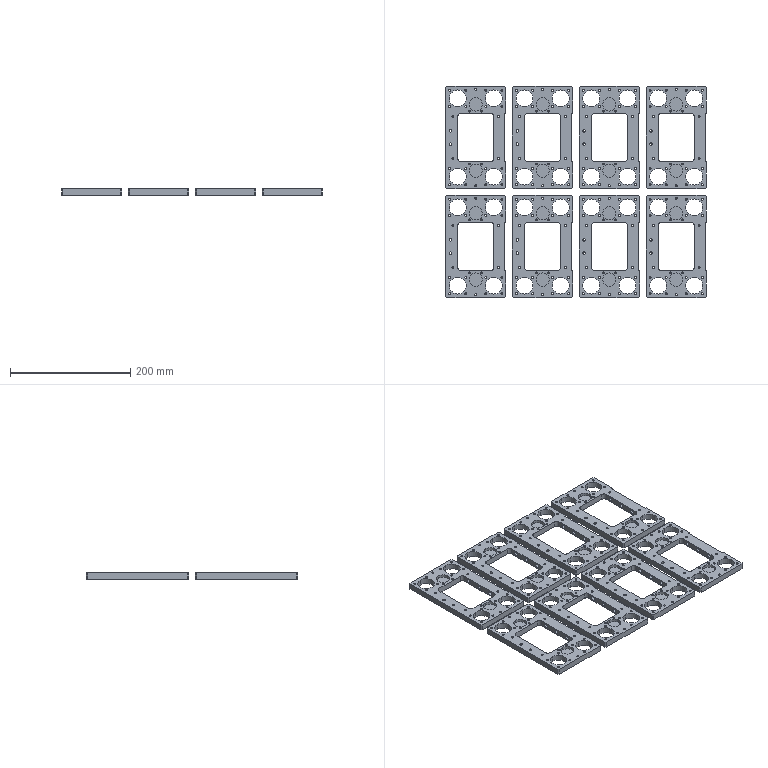NC program | NX | posted with a generic post | part box 433 x 351 x 10 mm
Lines 1 to 529 of 15742:
N10 G17 G21 G94 G90
(DRILLING , TOOL : D6A45)
N12 T01 M6
N14 G54
N16 G17 G0 G90 X-17.5 Y-55.5 B0. C0. S5000 M3
N18 G43 Z30. H1
N20 G94 G81 G98 Z-1. F350. R3.
N22 X-12.065 Y-38.935
N24 X-25.5 Y-25.5
N26 X-12.065 Y-12.065
N28 Y12.065
N30 X12.065
N32 Y-12.065
N34 X38.935
N36 Y12.065
N38 X55.5 Y10.5
N40 X72.065 Y12.065
N42 X85.5 Y25.5
N44 X72.065 Y38.935
N46 X65.5 Y46.5
N48 X55.5 Y35.5
N50 X45.5 Y46.5
N52 X38.935 Y38.935
N54 X25.5 Y25.5
N56 X12.065 Y38.935
N58 X-12.065
N60 X-17.5 Y55.5
N62 X17.5
N64 X13.5 Y79.5
N66 Y101.5
N68 X-17.5 Y125.5
N70 X-12.065 Y142.065
N72 X-25.5 Y155.5
N74 X-38.935 Y142.065
N76 X-45.5 Y134.5
N78 X-55.5 Y145.5
N80 X-65.5 Y134.5
N82 X-72.065 Y142.065
N84 Y168.935
N86 X-55.5 Y170.5
N88 X-38.935 Y168.935
N90 X-12.065
N92 X12.065
N94 X25.5 Y155.5
N96 X12.065 Y142.065
N98 X17.5 Y125.5
N100 X45.5 Y134.5
N102 X38.935 Y142.065
N104 Y168.935
N106 X55.5 Y170.5
N108 X72.065 Y168.935
N110 X55.5 Y145.5
N112 X65.5 Y134.5
N114 X72.065 Y142.065
N116 X93.5 Y125.5
N118 X98.935 Y142.065
N120 X85.5 Y155.5
N122 X98.935 Y168.935
N124 X123.065
N126 X149.935
N128 X166.5 Y170.5
N130 X183.065 Y168.935
N132 X196.5 Y155.5
N134 X209.935 Y168.935
N136 Y142.065
N138 X204.5 Y125.5
N140 X183.065 Y142.065
N142 X176.5 Y134.5
N144 X166.5 Y145.5
N146 X156.5 Y134.5
N148 X149.935 Y142.065
N150 X136.5 Y155.5
N152 X123.065 Y142.065
N154 X128.5 Y125.5
N156 X124.5 Y101.5
N158 Y79.5
N160 X128.5 Y55.5
N162 X123.065 Y38.935
N164 X93.5 Y55.5
N166 X98.935 Y38.935
N168 Y12.065
N170 X123.065
N172 X136.5 Y25.5
N174 X149.935 Y38.935
N176 X156.5 Y46.5
N178 X166.5 Y35.5
N180 X176.5 Y46.5
N182 X183.065 Y38.935
N184 X204.5 Y55.5
N186 X209.935 Y38.935
N188 X196.5 Y25.5
N190 X183.065 Y12.065
N192 X209.935
N194 Y-12.065
N196 X196.5 Y-25.5
N198 X209.935 Y-38.935
N200 X204.5 Y-55.5
N202 X183.065 Y-38.935
N204 X176.5 Y-46.5
N206 X166.5 Y-35.5
N208 X156.5 Y-46.5
N210 X149.935 Y-38.935
N212 X166.5 Y-10.5
N214 X183.065 Y-12.065
N216 X166.5 Y10.5
N218 X149.935 Y12.065
N220 Y-12.065
N222 X136.5 Y-25.5
N224 X123.065 Y-12.065
N226 X98.935
N228 X85.5 Y-25.5
N230 X72.065 Y-12.065
N232 X55.5 Y-10.5
N234 Y-35.5
N236 X72.065 Y-38.935
N238 X65.5 Y-46.5
N240 X45.5
N242 X38.935 Y-38.935
N244 X25.5 Y-25.5
N246 X12.065 Y-38.935
N248 X17.5 Y-55.5
N250 X13.5 Y-79.5
N252 Y-101.5
N254 X17.5 Y-125.5
N256 X12.065 Y-142.065
N258 X-12.065
N260 X-17.5 Y-125.5
N262 X-38.935 Y-142.065
N264 X-45.5 Y-134.5
N266 X-55.5 Y-145.5
N268 X-65.5 Y-134.5
N270 X-72.065 Y-142.065
N272 X-98.935
N274 X-93.5 Y-125.5
N276 X-97.5 Y-101.5
N278 Y-79.5
N280 X-93.5 Y-55.5
N282 X-98.935 Y-38.935
N284 X-85.5 Y-25.5
N286 X-72.065 Y-38.935
N288 X-65.5 Y-46.5
N290 X-55.5 Y-35.5
N292 X-45.5 Y-46.5
N294 X-38.935 Y-38.935
N296 Y-12.065
N298 X-55.5 Y-10.5
N300 X-72.065 Y-12.065
N302 Y12.065
N304 X-55.5 Y10.5
N306 X-38.935 Y12.065
N308 X-25.5 Y25.5
N310 X-38.935 Y38.935
N312 X-45.5 Y46.5
N314 X-55.5 Y35.5
N316 X-65.5 Y46.5
N318 X-72.065 Y38.935
N320 X-85.5 Y25.5
N322 X-98.935 Y12.065
N324 Y-12.065
N326 X-123.065
N328 Y12.065
N330 X-136.5 Y25.5
N332 X-149.935 Y12.065
N334 X-166.5 Y10.5
N336 Y35.5
N338 X-183.065 Y38.935
N340 X-176.5 Y46.5
N342 X-156.5
N344 X-149.935 Y38.935
N346 X-128.5 Y55.5
N348 X-123.065 Y38.935
N350 X-98.935
N352 X-93.5 Y55.5
N354 X-97.5 Y79.5
N356 Y101.5
N358 X-93.5 Y125.5
N360 X-98.935 Y142.065
N362 X-85.5 Y155.5
N364 X-98.935 Y168.935
N366 X-123.065
N368 Y142.065
N370 X-128.5 Y125.5
N372 X-156.5 Y134.5
N374 X-176.5
N376 X-183.065 Y142.065
N378 X-166.5 Y145.5
N380 X-149.935 Y142.065
N382 X-136.5 Y155.5
N384 X-149.935 Y168.935
N386 X-166.5 Y170.5
N388 X-183.065 Y168.935
N390 X-196.5 Y155.5
N392 X-209.935 Y168.935
N394 Y142.065
N396 X-204.5 Y125.5
N398 X-208.5 Y101.5
N400 Y79.5
N402 X-204.5 Y55.5
N404 X-209.935 Y38.935
N406 Y12.065
N408 X-196.5 Y25.5
N410 X-183.065 Y12.065
N412 Y-12.065
N414 X-166.5 Y-10.5
N416 X-149.935 Y-12.065
N418 X-136.5 Y-25.5
N420 X-123.065 Y-38.935
N422 X-128.5 Y-55.5
N424 X-149.935 Y-38.935
N426 X-156.5 Y-46.5
N428 X-166.5 Y-35.5
N430 X-176.5 Y-46.5
N432 X-183.065 Y-38.935
N434 X-196.5 Y-25.5
N436 X-209.935 Y-12.065
N438 Y-38.935
N440 X-204.5 Y-55.5
N442 X-208.5 Y-79.5
N444 Y-101.5
N446 X-204.5 Y-125.5
N448 X-209.935 Y-142.065
N450 Y-168.935
N452 X-196.5 Y-155.5
N454 X-183.065 Y-168.935
N456 X-166.5 Y-170.5
N458 X-183.065 Y-142.065
N460 X-176.5 Y-134.5
N462 X-166.5 Y-145.5
N464 X-156.5 Y-134.5
N466 X-149.935 Y-142.065
N468 X-128.5 Y-125.5
N470 X-123.065 Y-142.065
N472 X-136.5 Y-155.5
N474 X-149.935 Y-168.935
N476 X-123.065
N478 X-98.935
N480 X-85.5 Y-155.5
N482 X-72.065 Y-168.935
N484 X-55.5 Y-170.5
N486 X-38.935 Y-168.935
N488 X-25.5 Y-155.5
N490 X-12.065 Y-168.935
N492 X12.065
N494 X25.5 Y-155.5
N496 X38.935 Y-142.065
N498 X45.5 Y-134.5
N500 X55.5 Y-145.5
N502 X38.935 Y-168.935
N504 X55.5 Y-170.5
N506 X72.065 Y-168.935
N508 X65.5 Y-134.5
N510 X72.065 Y-142.065
N512 X85.5 Y-155.5
N514 X98.935 Y-168.935
N516 X123.065
N518 X149.935
N520 X166.5 Y-170.5
N522 X183.065 Y-168.935
N524 X209.935
N526 X196.5 Y-155.5
N528 X209.935 Y-142.065
N530 X204.5 Y-125.5
N532 X183.065 Y-142.065
N534 X176.5 Y-134.5
N536 X166.5 Y-145.5
N538 X156.5 Y-134.5
N540 X149.935 Y-142.065
N542 X136.5 Y-155.5
N544 X123.065 Y-142.065
N546 X98.935
N548 X93.5 Y-125.5
N550 X128.5
N552 X124.5 Y-101.5
N554 Y-79.5
N556 X128.5 Y-55.5
N558 X123.065 Y-38.935
N560 X98.935
N562 X93.5 Y-55.5
N564 G80
N566 G0 X93.5 Y-55.5 Z30.
N568 M5
(DRILLING_COPY , TOOL : 3.3ZT)
N570 T03 M6
N572 G54
N574 G17 G0 G90 X-209.935 Y168.935 B0. C0. S2000 M3
N576 G43 Z30. H3
N578 G94 G83 G98 Z-12.491 F200. Q2. R3.
N580 X-183.065
N582 X-166.5 Y170.5
N584 X-149.935 Y168.935
N586 X-123.065
N588 X-98.935
N590 X-72.065
N592 X-55.5 Y170.5
N594 X-38.935 Y168.935
N596 X-12.065
N598 X12.065
N600 X38.935
N602 X55.5 Y170.5
N604 X72.065 Y168.935
N606 X98.935
N608 X123.065
N610 X149.935
N612 X166.5 Y170.5
N614 X183.065 Y168.935
N616 X209.935
N618 Y142.065
N620 X204.5 Y125.5
N622 X183.065 Y142.065
N624 X176.5 Y134.5
N626 X156.5
N628 X149.935 Y142.065
N630 X128.5 Y125.5
N632 X123.065 Y142.065
N634 X98.935
N636 X93.5 Y125.5
N638 X72.065 Y142.065
N640 X65.5 Y134.5
N642 X45.5
N644 X38.935 Y142.065
N646 X17.5 Y125.5
N648 X12.065 Y142.065
N650 X-12.065
N652 X-17.5 Y125.5
N654 X-38.935 Y142.065
N656 X-45.5 Y134.5
N658 X-65.5
N660 X-72.065 Y142.065
N662 X-93.5 Y125.5
N664 X-98.935 Y142.065
N666 X-123.065
N668 X-128.5 Y125.5
N670 X-149.935 Y142.065
N672 X-156.5 Y134.5
N674 X-176.5
N676 X-183.065 Y142.065
N678 X-209.935
N680 X-204.5 Y125.5
N682 X-176.5 Y46.5
N684 X-183.065 Y38.935
N686 X-204.5 Y55.5
N688 X-209.935 Y38.935
N690 Y12.065
N692 Y-12.065
N694 Y-38.935
N696 X-204.5 Y-55.5
N698 X-183.065 Y-38.935
N700 X-176.5 Y-46.5
N702 X-156.5
N704 X-149.935 Y-38.935
N706 Y-12.065
N708 X-166.5 Y-10.5
N710 X-183.065 Y-12.065
N712 Y12.065
N714 X-166.5 Y10.5
N716 X-149.935 Y12.065
N718 Y38.935
N720 X-156.5 Y46.5
N722 X-128.5 Y55.5
N724 X-123.065 Y38.935
N726 Y12.065
N728 X-98.935
N730 X-72.065 Y-12.065
N732 X-55.5 Y-10.5
N734 X-38.935 Y-12.065
N736 Y12.065
N738 X-55.5 Y10.5
N740 X-72.065 Y12.065
N742 X-98.935 Y38.935
N744 X-93.5 Y55.5
N746 X-72.065 Y38.935
N748 X-65.5 Y46.5
N750 X-45.5
N752 X-38.935 Y38.935
N754 X-17.5 Y55.5
N756 X-12.065 Y38.935
N758 Y12.065
N760 X12.065
N762 Y38.935
N764 X17.5 Y55.5
N766 X38.935 Y38.935
N768 X45.5 Y46.5
N770 X65.5
N772 X72.065 Y38.935
N774 X93.5 Y55.5
N776 X98.935 Y38.935
N778 X123.065
N780 X128.5 Y55.5
N782 X149.935 Y38.935
N784 X156.5 Y46.5
N786 X176.5
N788 X183.065 Y38.935
N790 X204.5 Y55.5
N792 X209.935 Y38.935
N794 Y12.065
N796 Y-12.065
N798 Y-38.935
N800 X204.5 Y-55.5
N802 X183.065 Y-38.935
N804 X176.5 Y-46.5
N806 X156.5
N808 X149.935 Y-38.935
N810 Y-12.065
N812 X166.5 Y-10.5
N814 X183.065 Y-12.065
N816 Y12.065
N818 X166.5 Y10.5
N820 X149.935 Y12.065
N822 X123.065
N824 Y-12.065
N826 Y-38.935
N828 X128.5 Y-55.5
N830 X98.935 Y-38.935
N832 X93.5 Y-55.5
N834 X72.065 Y-38.935
N836 X65.5 Y-46.5
N838 X45.5
N840 X38.935 Y-38.935
N842 Y-12.065
N844 X55.5 Y-10.5
N846 X72.065 Y-12.065
N848 X98.935
N850 Y12.065
N852 X72.065
N854 X55.5 Y10.5
N856 X38.935 Y12.065
N858 X12.065 Y-12.065
N860 X-12.065
N862 X12.065 Y-38.935
N864 X17.5 Y-55.5
N866 X-12.065 Y-38.935
N868 X-17.5 Y-55.5
N870 X-38.935 Y-38.935
N872 X-45.5 Y-46.5
N874 X-65.5
N876 X-72.065 Y-38.935
N878 X-93.5 Y-55.5
N880 X-98.935 Y-38.935
N882 Y-12.065
N884 X-123.065
N886 Y-38.935
N888 X-128.5 Y-55.5
N890 Y-125.5
N892 X-123.065 Y-142.065
N894 X-98.935
N896 X-93.5 Y-125.5
N898 X-72.065 Y-142.065
N900 X-65.5 Y-134.5
N902 X-45.5
N904 X-38.935 Y-142.065
N906 X-17.5 Y-125.5
N908 X-12.065 Y-142.065
N910 X12.065
N912 X17.5 Y-125.5
N914 X38.935 Y-142.065
N916 X45.5 Y-134.5
N918 X65.5
N920 X72.065 Y-142.065
N922 X93.5 Y-125.5
N924 X98.935 Y-142.065
N926 X123.065
N928 X128.5 Y-125.5
N930 X149.935 Y-142.065
N932 X156.5 Y-134.5
N934 X176.5
N936 X183.065 Y-142.065
N938 X204.5 Y-125.5
N940 X209.935 Y-142.065
N942 Y-168.935
N944 X183.065
N946 X166.5 Y-170.5
N948 X149.935 Y-168.935
N950 X123.065
N952 X98.935
N954 X72.065
N956 X55.5 Y-170.5
N958 X38.935 Y-168.935
N960 X12.065
N962 X-12.065
N964 X-38.935
N966 X-55.5 Y-170.5
N968 X-72.065 Y-168.935
N970 X-98.935
N972 X-123.065
N974 X-149.935
N976 X-166.5 Y-170.5
N978 X-183.065 Y-168.935
N980 X-209.935
N982 Y-142.065
N984 X-204.5 Y-125.5
N986 X-183.065 Y-142.065
N988 X-176.5 Y-134.5
N990 X-156.5
N992 X-149.935 Y-142.065
N994 G80
N996 G0 X-149.935 Y-142.065 Z30.
N998 M5
(DRILLING_COPY_COPY , TOOL : 4.2ZT)
N1000 T04 M6
N1002 G54
N1004 G17 G0 G90 X124.5 Y-79.5 B0. C0. S2000 M3
N1006 G43 Z30. H4
N1008 G94 G83 G98 Z-12.762 F300. Q2. R3.
N1010 Y-101.5
N1012 X13.5
N1014 Y-79.5
N1016 X-97.5
N1018 Y-101.5
N1020 X-208.5
N1022 Y-79.5
N1024 Y79.5
N1026 Y101.5
N1028 X-97.5
N1030 Y79.5
N1032 X13.5
N1034 Y101.5
N1036 X124.5
N1038 Y79.5
N1040 G80
N1042 G0 X124.5 Y79.5 Z30.
N1044 M5